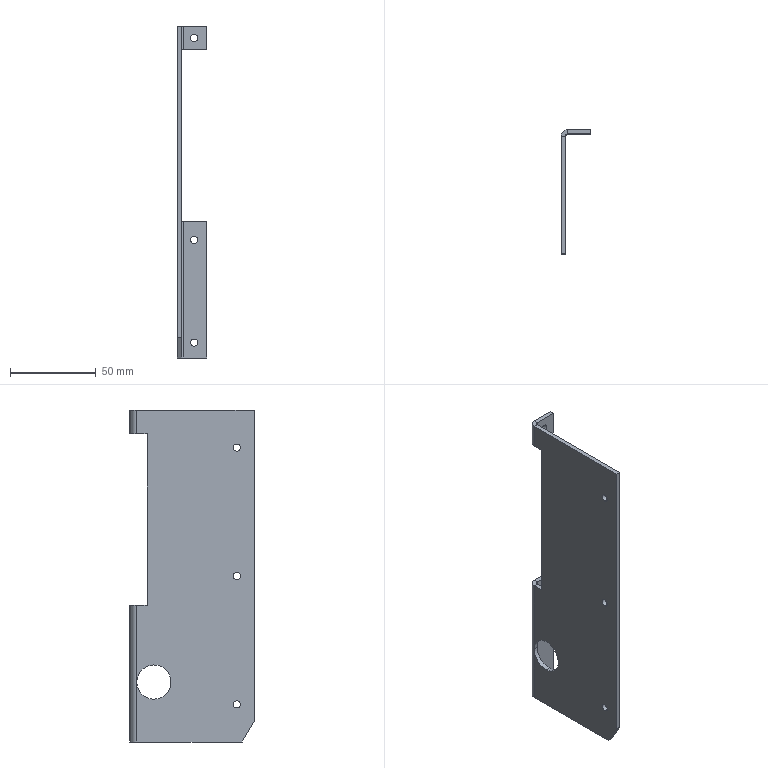Part | STEP file | 64605526 | 1 solid | 42 faces | box 17.5 x 72.5 x 194 mm | volume 34813 mm3 | plane 23 | cylinder 19 | commonest cylinder face diameters 4.2 x12 20 x3 3 x2 8 x2